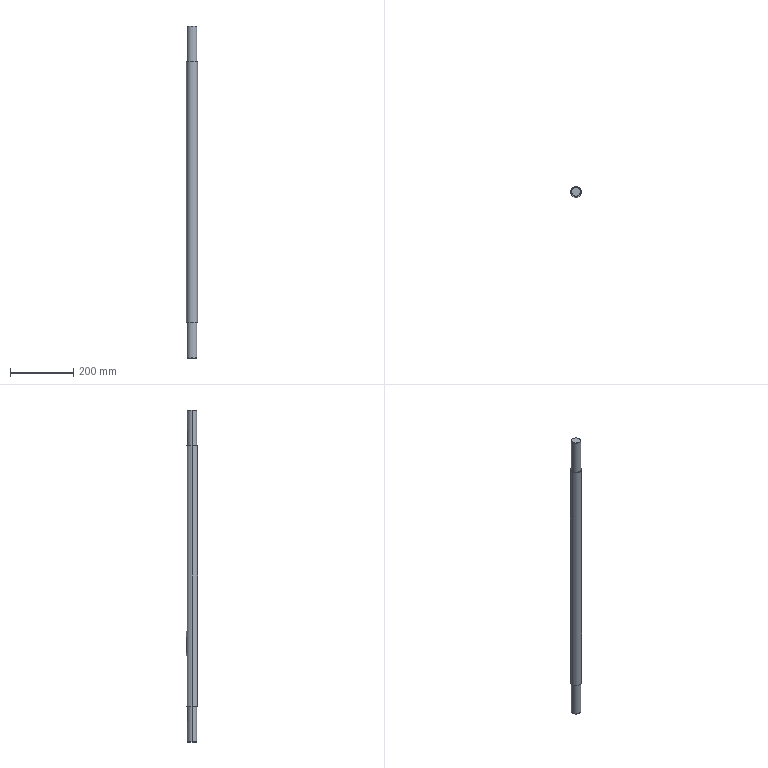Part | STEP file | 1 solid | 32 faces | box 35 x 35 x 1052 mm | volume 947063 mm3 | cylinder 15 | plane 13 | cone 4 | commonest cylinder face diameters 10 x9 30 x4 35 x2